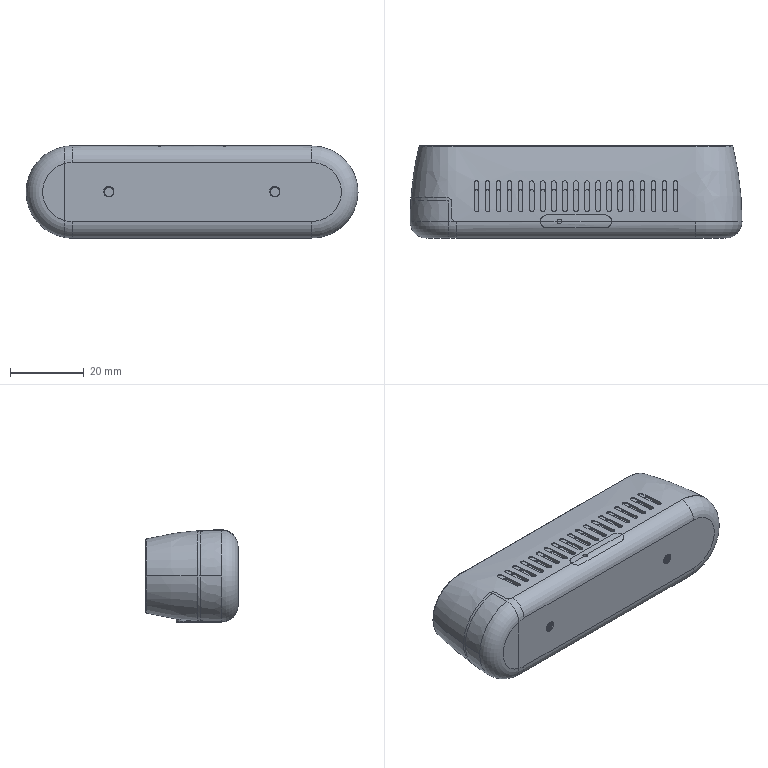Part | SolidWorks | features ICE 13, SweepThread 3, Fillet 2, Split 2, Blend 1 | 5 solids | 382 faces | box 90 x 25 x 25 mm | volume 48696 mm3 | cylinder 178 | plane 154 | spline 40 | torus 10 | commonest cylinder face diameters 1.25 x107 2.5 x34 5 x11 3.5 x7 9 x5 2.4 x4